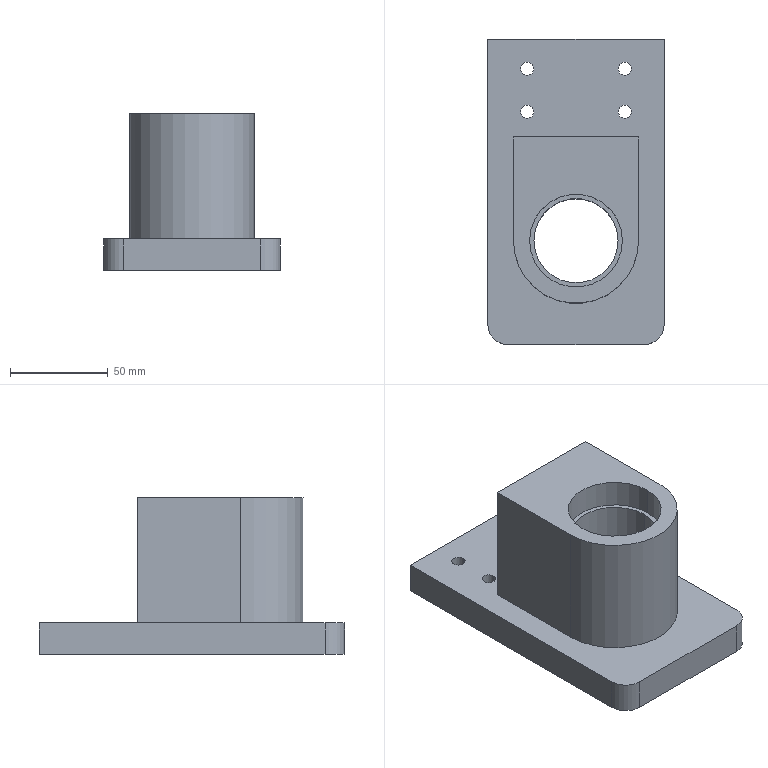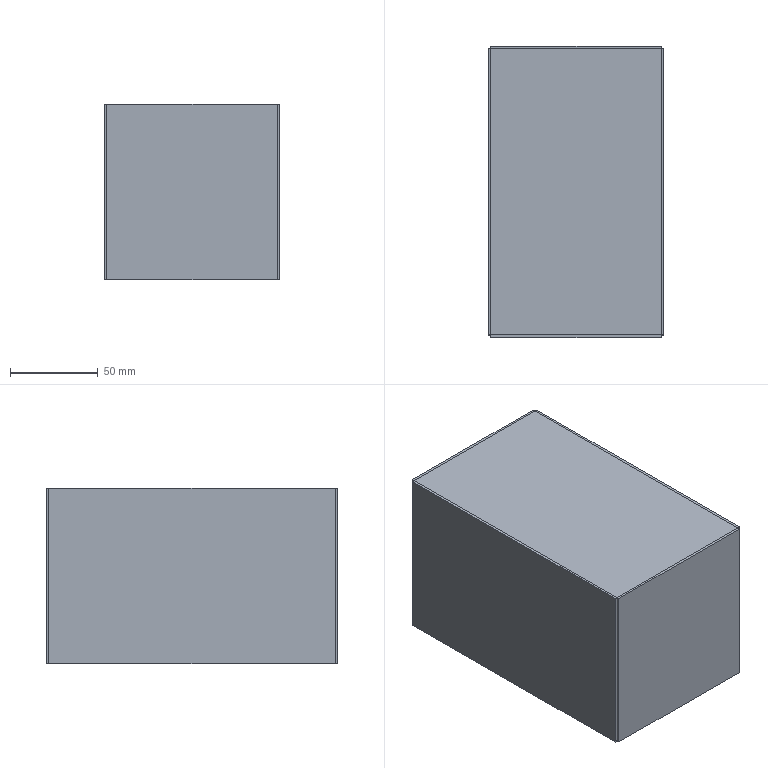CAM job | NX | 3-axis milling, drilling | part box 90 x 156 x 80 mm | stock box 100 x 166 x 100 mm
Tools:
number,name,description,diameter,corner_radius,flute_length,length,flutes
0,D10-30-D10-75-3T-FINISH,D10-30-D10-75-3T,10.0,0.0,30.0,75.0,3
5,D12-36-D12-120-3T-FINISH,D12-55-D12-120-3T,12.0,0.0,55.0,120.0,3
2,D16-48-D16-100-3T-FINISH,D16-48-D16-100-3T,16.0,0.0,48.0,100.0,3
0,刀杆C25-D25-150-2T,刀杆C25-D25-150-2T,25.0,0.8,80.0,150.0,2
3,D50面刀,D50面刀,50.0,0.0,30.0,30.0,4
0,钻头D6.8-73-105,钻刀D6.8-73-105,6.8,0.0,73.0,105.0,2
0,上排M8-28-D6.2-70,上排M8-28-D6.2-70,8.0,0.0,28.0,33.0,2
4,倒角D10-90度,倒角D10-90度,10.0,0.0,10.0,75.0,2
Operations:
program,operation,operation_type,tool,method,geometry_group,spindle_rpm,surface_speed,feed_per_tooth,feed_cut,feed_plunge,cut_length_mm,path_length_mm,cut_time_min,machine_time_min
A1,CAVITY_MILL_COPY,CavityMilling,刀杆C25-D25-150-2T,METHOD,WORKPIECE_54,2000.0,100.0,0.75,3000.0,100.0,108966.328,127597.198,36.322,38.185
A1,PLANAR_MILL,PlanarMilling,D50面刀,METHOD,A-G54,2000.0,314.0,0.075,600.0,100.0,504.0,859.822,0.84,0.8756
A1,CAVITY_MILL,CavityMilling,刀杆C25-D25-150-2T,METHOD,WORKPIECE_54,2000.0,100.0,0.75,3000.0,100.0,86813.543,110617.468,28.938,31.318
A1,PLANAR_MILL_3,PlanarMilling,D16-48-D16-100-3T-FINISH,METHOD,A-G54,2000.0,100.0,0.1,600.0,100.0,1429.431,1611.431,2.382,2.401
A1,PLANAR_MILL_1,PlanarMilling,D16-48-D16-100-3T-FINISH,METHOD,WORKPIECE_54,2000.0,314.0,0.075,600.0,100.0,1988.667,2420.666,3.314,3.358
A1,PLANAR_MILL_1_COPY,PlanarMilling,D16-48-D16-100-3T-FINISH,METHOD,WORKPIECE_54,2000.0,314.0,0.075,600.0,100.0,1088.559,1306.559,1.814,1.836
A1,PLANAR_MILL_2,PlanarMilling,D16-48-D16-100-3T-FINISH,METHOD,WORKPIECE_54,2000.0,314.0,0.075,600.0,100.0,218.153,302.153,0.3636,0.372
A1,PLANAR_MILL_2_COPY,PlanarMilling,D16-48-D16-100-3T-FINISH,METHOD,WORKPIECE_54,2000.0,314.0,0.075,600.0,100.0,569.812,1045.815,0.9497,0.9973
A1,PLANAR_MILL_4,PlanarMilling,倒角D10-90度,METHOD,A-G54,3000.0,94.0,0.1333,800.0,100.0,147.145,207.145,0.1839,0.1899
A1,PLANAR_MILL_4_COPY,PlanarMilling,倒角D10-90度,METHOD,A-G54,3000.0,94.0,0.1333,800.0,100.0,293.38,353.38,0.3667,0.3727
A1,PLANAR_MILL_4_COPY_1,PlanarMilling,倒角D10-90度,METHOD,A-G54,3000.0,94.0,0.1333,800.0,100.0,120.498,212.498,0.1506,0.1598
B1,ADAPTIVE_MILLING,CavityMilling,D12-36-D12-120-3T-FINISH,METHOD,WORKPIECE_55,3000.0,113.0,0.2222,2000.0,100.0,27286.388,27339.988,13.643,13.649
B1,PLANAR_MILL_5,PlanarMilling,D12-36-D12-120-3T-FINISH,METHOD,WORKPIECE_55,3000.0,113.0,0.1111,1000.0,100.0,574.891,658.691,0.5749,0.5833
B1,FLOOR_WALL,VolumeBased25DMillingOperation,D50面刀,METHOD,WORKPIECE_55,2000.0,314.0,0.075,600.0,100.0,722.575,776.575,1.204,1.21
B1,PLANAR_MILL_5_COPY,PlanarMilling,D10-30-D10-75-3T-FINISH,METHOD,WORKPIECE_55,3000.0,94.0,0.1111,1000.0,100.0,256.425,340.425,0.2564,0.2648
B1,PLANAR_MILL_6,PlanarMilling,倒角D10-90度,METHOD,WORKPIECE_55,3000.0,94.0,0.1667,1000.0,100.0,506.265,566.265,0.5063,0.5123
B1,PLANAR_MILL_6_COPY,PlanarMilling,倒角D10-90度,METHOD,WORKPIECE_55,3000.0,94.0,0.1667,1000.0,100.0,147.145,207.145,0.1471,0.1531
B1,PLANAR_MILL_6_COPY_1,PlanarMilling,倒角D10-90度,METHOD,WORKPIECE_55,3000.0,94.0,0.1667,1000.0,100.0,120.498,212.498,0.1205,0.1297
B1,DRILLING,Operation,倒角D10-90度,METHOD,WORKPIECE_55,1200.0,37.0,0.0417,100.0,0.0,18.0,199.497,0.18,0.1981
B1,DRILLING_COPY,Operation,钻头D6.8-73-105,METHOD,WORKPIECE_55,1200.0,25.0,0.0417,100.0,0.0,92.0,347.497,0.92,0.9455
B1,DRILLING_COPY_1,Operation,倒角D10-90度,METHOD,WORKPIECE_55,1200.0,37.0,0.0417,100.0,0.0,28.0,219.497,0.28,0.2991
B1,DRILLING_COPY_COPY,Operation,上排M8-28-D6.2-70,METHOD,WORKPIECE_55,300.0,7.0,0.625,375.0,0.0,52.0,267.497,0.1387,0.1602